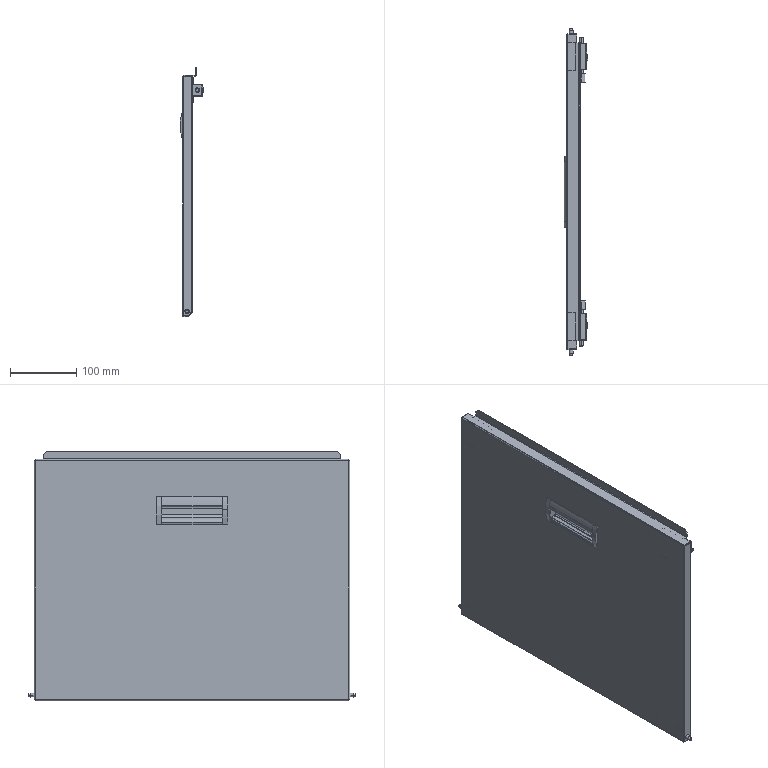Part | SolidWorks | 16 solids | 429 faces | box 35.649 x 494 x 376.5 mm | volume 364955 mm3 | plane 243 | cylinder 174 | cone 8 | torus 4 | commonest cylinder face diameters 1 x18 2.5 x16 3.2 x16 0.6 x14 7 x13 2 x8